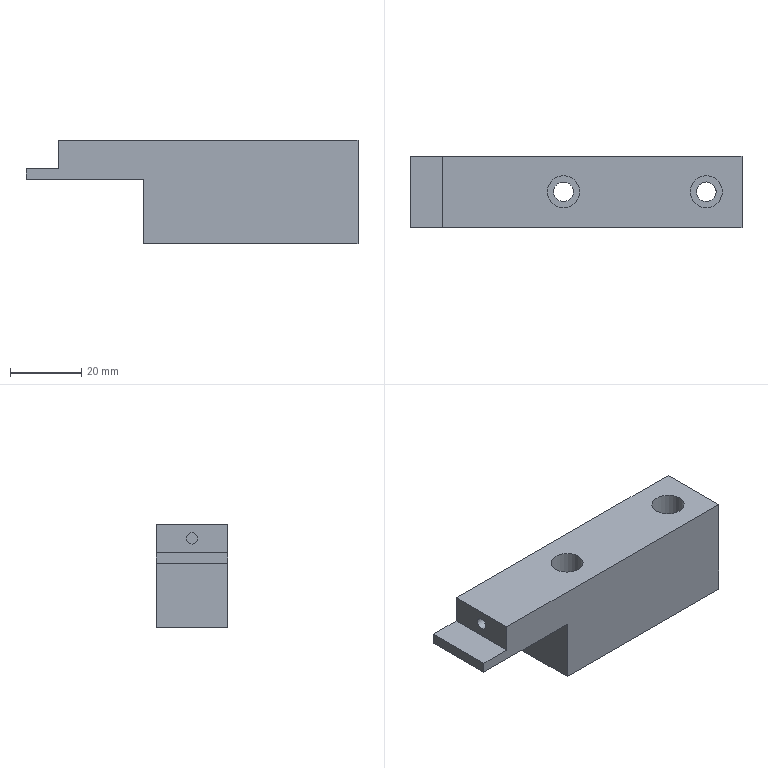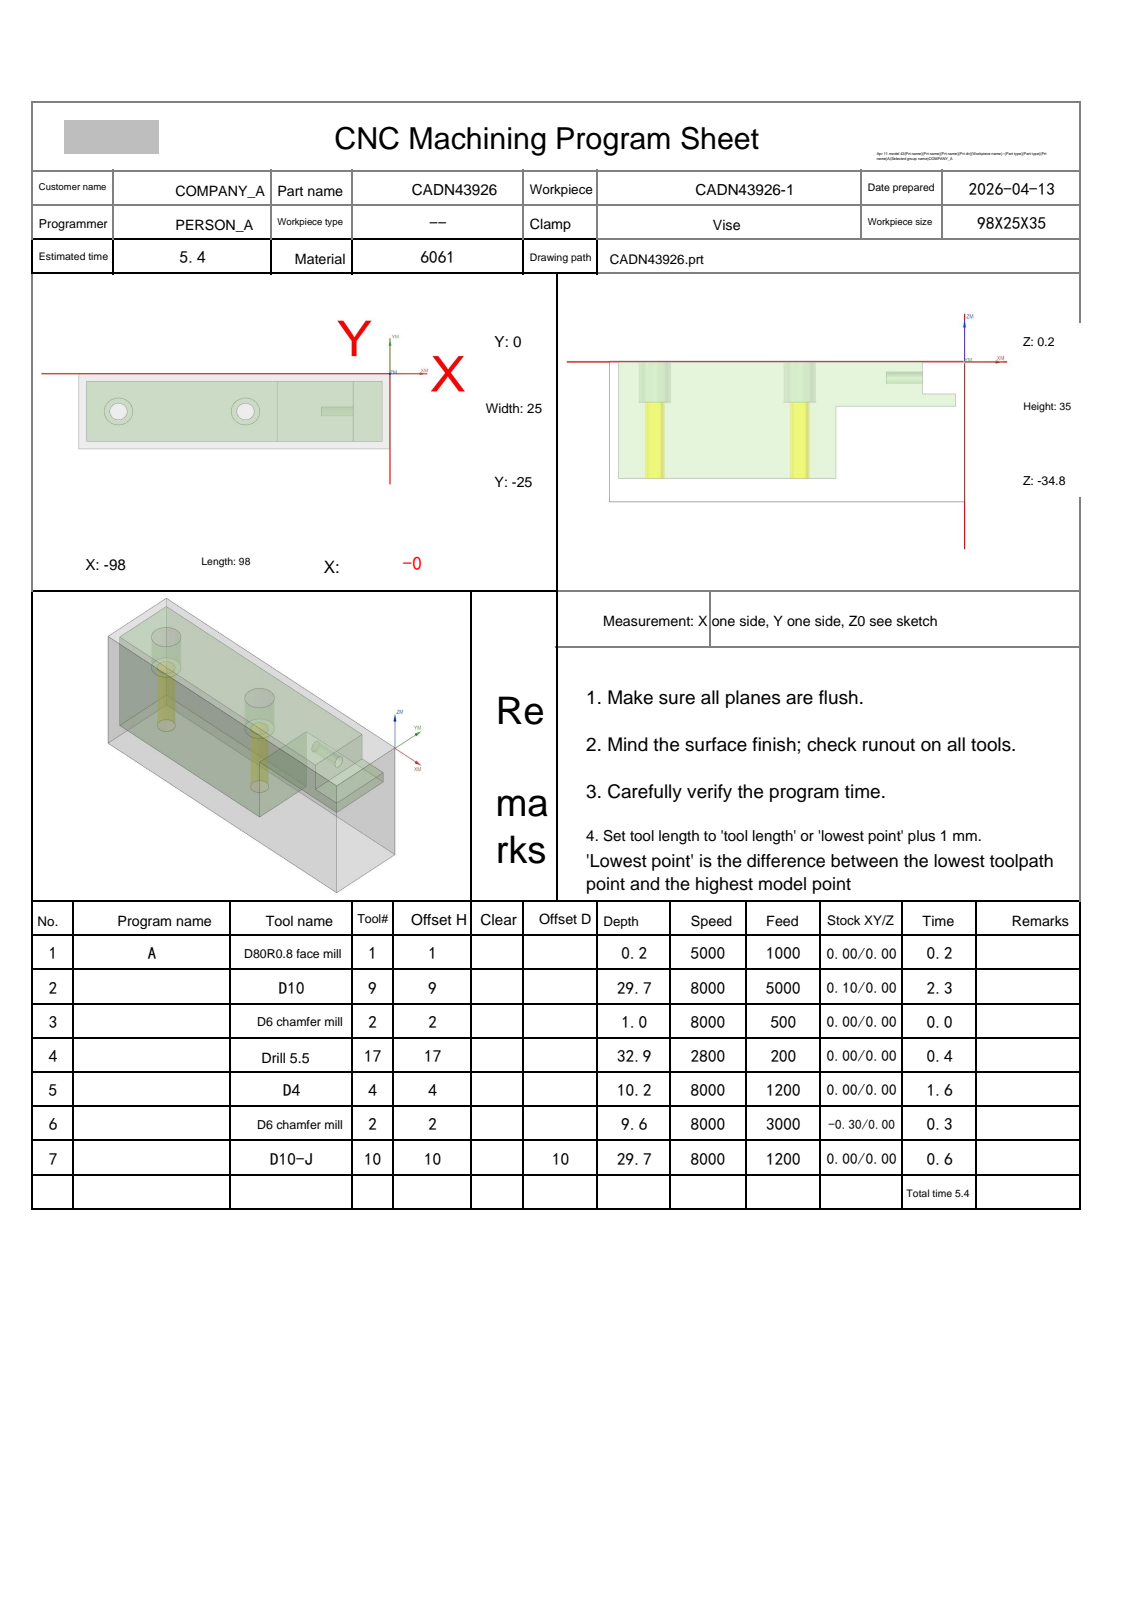NC program | NX | posted by the shop | part box 93 x 20 x 29 mm
Whole program:
%
O0001
(Machine time: 6.75 MIN)
(===Total Tool:6===)
(T1=D80R0.8 face mill D=80.  R=0.8  D-  H01 Z=0.    )
(T9=D10     D=10.  R=0.   D-  H09 Z=-29.5 )
(T2=D6 chamfer mill   D=6.   R=0.   D-  H02 Z=-9.45 )
(T17=drill 5.5  D=5.5  DR_a=118 D-  H17 Z=-32.65)
(T4=D4      D=4.   R=0.   D4  H04 Z=-10.  )
(T10=D10-J  D=10.  R=0.   D10 H10 Z=-29.5 )
G80 G90 G17 G49 G40
G91 G28 Z0
M01
N1 T01 M06
(D80R0.8 face mill  D=80. R=0.8 H=01 ce=0.00 di=0.00)
G00 G90 G54 X42.5 Y-12.5 M03 S5000
G43 H01 Z20.
M08
Z2.
G01 Z0.0 F1000.
X37.5
X-135.5
X-140.5
Z2.
G00 Z20.
G91 G28 Z0.0
M05
M09
G91 G28 Z0.0
M01
N2 T09 M06
(D10  D=10. R=0. H=09 ce=0.10 di=0.00)
G00 G90 G54 X-49. Y-27.6 M03 S8000
G43 H09 Z20.
M08
Z.5
G01 X-95.5 Z.358 F5000.
G02 X-100.6 Y-22.5 Z.333 I0.0 J5.1
G01 Y-2.5 Z.272
G02 X-95.5 Y2.6 Z.248 I5.1 J0.0
G01 X-2.5 Z-.037
G02 X2.6 Y-2.5 Z-.062 I0.0 J-5.1
G01 Y-22.5 Z-.123
G02 X-2.5 Y-27.6 Z-.147 I-5.1 J0.0
G01 X-95.5 Z-.432
G02 X-100.6 Y-22.5 Z-.456 I0.0 J5.1
G01 Y-2.5 Z-.517
G02 X-95.5 Y2.6 Z-.542 I5.1 J0.0
G01 X-2.5 Z-.826
G02 X2.6 Y-2.5 Z-.851 I0.0 J-5.1
G01 Y-22.5 Z-.912
G02 X-2.5 Y-27.6 Z-.937 I-5.1 J0.0
G01 X-95.5 Z-1.221
G02 X-100.6 Y-22.5 Z-1.246 I0.0 J5.1
G01 Y-2.5 Z-1.307
G02 X-95.5 Y2.6 Z-1.331 I5.1 J0.0
G01 X-2.5 Z-1.616
G02 X2.6 Y-2.5 Z-1.64 I0.0 J-5.1
G01 Y-22.5 Z-1.702
G02 X-2.5 Y-27.6 Z-1.726 I-5.1 J0.0
G01 X-95.5 Z-2.011
G02 X-100.6 Y-22.5 Z-2.035 I0.0 J5.1
G01 Y-2.5 Z-2.096
G02 X-95.5 Y2.6 Z-2.121 I5.1 J0.0
G01 X-2.5 Z-2.405
G02 X2.6 Y-2.5 Z-2.43 I0.0 J-5.1
G01 Y-22.5 Z-2.491
G02 X-2.5 Y-27.6 Z-2.516 I-5.1 J0.0
G01 X-95.5 Z-2.8
G02 X-100.6 Y-22.5 Z-2.825 I0.0 J5.1
G01 Y-2.5 Z-2.886
G02 X-95.5 Y2.6 Z-2.91 I5.1 J0.0
G01 X-2.5 Z-3.195
G02 X2.6 Y-2.5 Z-3.219 I0.0 J-5.1
G01 Y-22.5 Z-3.281
G02 X-2.5 Y-27.6 Z-3.305 I-5.1 J0.0
G01 X-95.5 Z-3.59
G02 X-100.6 Y-22.5 Z-3.614 I0.0 J5.1
G01 Y-2.5 Z-3.675
G02 X-95.5 Y2.6 Z-3.7 I5.1 J0.0
G01 X-2.5 Z-3.984
G02 X2.6 Y-2.5 Z-4.009 I0.0 J-5.1
G01 Y-22.5 Z-4.07
G02 X-2.5 Y-27.6 Z-4.095 I-5.1 J0.0
G01 X-95.5 Z-4.379
G02 X-100.6 Y-22.5 Z-4.404 I0.0 J5.1
G01 Y-2.5 Z-4.465
G02 X-95.5 Y2.6 Z-4.489 I5.1 J0.0
G01 X-2.5 Z-4.774
G02 X2.6 Y-2.5 Z-4.798 I0.0 J-5.1
G01 Y-22.5 Z-4.86
G02 X-2.5 Y-27.6 Z-4.884 I-5.1 J0.0
G01 X-95.5 Z-5.169
G02 X-100.6 Y-22.5 Z-5.193 I0.0 J5.1
G01 Y-2.5 Z-5.254
G02 X-95.5 Y2.6 Z-5.279 I5.1 J0.0
G01 X-2.5 Z-5.563
G02 X2.6 Y-2.5 Z-5.588 I0.0 J-5.1
G01 Y-22.5 Z-5.649
G02 X-2.5 Y-27.6 Z-5.674 I-5.1 J0.0
G01 X-95.5 Z-5.958
G02 X-100.6 Y-22.5 Z-5.983 I0.0 J5.1
G01 Y-2.5 Z-6.044
G02 X-95.5 Y2.6 Z-6.068 I5.1 J0.0
G01 X-2.5 Z-6.353
G02 X2.6 Y-2.5 Z-6.377 I0.0 J-5.1
G01 Y-22.5 Z-6.438
G02 X-2.5 Y-27.6 Z-6.463 I-5.1 J0.0
G01 X-95.5 Z-6.748
G02 X-100.6 Y-22.5 Z-6.772 I0.0 J5.1
G01 Y-2.5 Z-6.833
G02 X-95.5 Y2.6 Z-6.858 I5.1 J0.0
G01 X-2.5 Z-7.142
G02 X2.6 Y-2.5 Z-7.167 I0.0 J-5.1
G01 Y-22.5 Z-7.228
G02 X-2.5 Y-27.6 Z-7.252 I-5.1 J0.0
G01 X-95.5 Z-7.537
G02 X-100.6 Y-22.5 Z-7.562 I0.0 J5.1
G01 Y-2.5 Z-7.623
G02 X-95.5 Y2.6 Z-7.647 I5.1 J0.0
G01 X-2.5 Z-7.932
G02 X2.6 Y-2.5 Z-7.956 I0.0 J-5.1
G01 Y-22.5 Z-8.017
G02 X-2.5 Y-27.6 Z-8.042 I-5.1 J0.0
G01 X-95.5 Z-8.326
G02 X-100.6 Y-22.5 Z-8.351 I0.0 J5.1
G01 Y-2.5 Z-8.412
G02 X-95.5 Y2.6 Z-8.437 I5.1 J0.0
G01 X-2.5 Z-8.721
G02 X2.6 Y-2.5 Z-8.746 I0.0 J-5.1
G01 Y-22.5 Z-8.807
G02 X-2.5 Y-27.6 Z-8.831 I-5.1 J0.0
G01 X-95.5 Z-9.116
G02 X-100.6 Y-22.5 Z-9.14 I0.0 J5.1
G01 Y-2.5 Z-9.202
G02 X-95.5 Y2.6 Z-9.226 I5.1 J0.0
G01 X-2.5 Z-9.511
G02 X2.6 Y-2.5 Z-9.535 I0.0 J-5.1
G01 Y-22.5 Z-9.596
G02 X-2.5 Y-27.6 Z-9.621 I-5.1 J0.0
G01 X-95.5 Z-9.905
G02 X-100.6 Y-22.5 Z-9.93 I0.0 J5.1
G01 Y-2.5 Z-9.991
G02 X-95.5 Y2.6 Z-10.016 I5.1 J0.0
G01 X-2.5 Z-10.3
G02 X2.6 Y-2.5 Z-10.325 I0.0 J-5.1
G01 Y-22.5 Z-10.386
G02 X-2.5 Y-27.6 Z-10.41 I-5.1 J0.0
G01 X-95.5 Z-10.695
G02 X-100.6 Y-22.5 Z-10.719 I0.0 J5.1
G01 Y-2.5 Z-10.781
G02 X-95.5 Y2.6 Z-10.805 I5.1 J0.0
G01 X-2.5 Z-11.09
G02 X2.6 Y-2.5 Z-11.114 I0.0 J-5.1
G01 Y-22.5 Z-11.175
G02 X-2.5 Y-27.6 Z-11.2 I-5.1 J0.0
G01 X-95.5 Z-11.484
G02 X-100.6 Y-22.5 Z-11.509 I0.0 J5.1
G01 Y-2.5 Z-11.57
G02 X-95.5 Y2.6 Z-11.595 I5.1 J0.0
G01 X-2.5 Z-11.879
G02 X2.6 Y-2.5 Z-11.904 I0.0 J-5.1
G01 Y-22.5 Z-11.965
G02 X-2.5 Y-27.6 Z-11.989 I-5.1 J0.0
G01 X-95.5 Z-12.274
G02 X-100.6 Y-22.5 Z-12.298 I0.0 J5.1
G01 Y-2.5 Z-12.36
G02 X-95.5 Y2.6 Z-12.384 I5.1 J0.0
G01 X-2.5 Z-12.669
G02 X2.6 Y-2.5 Z-12.693 I0.0 J-5.1
G01 Y-22.5 Z-12.754
G02 X-2.5 Y-27.6 Z-12.779 I-5.1 J0.0
G01 X-95.5 Z-13.063
G02 X-100.6 Y-22.5 Z-13.088 I0.0 J5.1
G01 Y-2.5 Z-13.149
G02 X-95.5 Y2.6 Z-13.174 I5.1 J0.0
G01 X-2.5 Z-13.458
G02 X2.6 Y-2.5 Z-13.483 I0.0 J-5.1
G01 Y-22.5 Z-13.544
G02 X-2.5 Y-27.6 Z-13.568 I-5.1 J0.0
G01 X-95.5 Z-13.853
G02 X-100.6 Y-22.5 Z-13.877 I0.0 J5.1
G01 Y-2.5 Z-13.938
G02 X-95.5 Y2.6 Z-13.963 I5.1 J0.0
G01 X-2.5 Z-14.248
G02 X2.6 Y-2.5 Z-14.272 I0.0 J-5.1
G01 Y-22.5 Z-14.333
G02 X-2.5 Y-27.6 Z-14.358 I-5.1 J0.0
G01 X-95.5 Z-14.642
G02 X-100.6 Y-22.5 Z-14.667 I0.0 J5.1
G01 Y-2.5 Z-14.728
G02 X-95.5 Y2.6 Z-14.752 I5.1 J0.0
G01 X-2.5 Z-15.037
G02 X2.6 Y-2.5 Z-15.062 I0.0 J-5.1
G01 Y-22.5 Z-15.123
G02 X-2.5 Y-27.6 Z-15.147 I-5.1 J0.0
G01 X-95.5 Z-15.432
G02 X-100.6 Y-22.5 Z-15.456 I0.0 J5.1
G01 Y-2.5 Z-15.517
G02 X-95.5 Y2.6 Z-15.542 I5.1 J0.0
G01 X-2.5 Z-15.826
G02 X2.6 Y-2.5 Z-15.851 I0.0 J-5.1
G01 Y-22.5 Z-15.912
G02 X-2.5 Y-27.6 Z-15.937 I-5.1 J0.0
G01 X-95.5 Z-16.221
G02 X-100.6 Y-22.5 Z-16.246 I0.0 J5.1
G01 Y-2.5 Z-16.307
G02 X-95.5 Y2.6 Z-16.331 I5.1 J0.0
G01 X-2.5 Z-16.616
G02 X2.6 Y-2.5 Z-16.64 I0.0 J-5.1
G01 Y-22.5 Z-16.702
G02 X-2.5 Y-27.6 Z-16.726 I-5.1 J0.0
G01 X-95.5 Z-17.011
G02 X-100.6 Y-22.5 Z-17.035 I0.0 J5.1
G01 Y-2.5 Z-17.096
G02 X-95.5 Y2.6 Z-17.121 I5.1 J0.0
G01 X-2.5 Z-17.405
G02 X2.6 Y-2.5 Z-17.43 I0.0 J-5.1
G01 Y-22.5 Z-17.491
G02 X-2.5 Y-27.6 Z-17.516 I-5.1 J0.0
G01 X-95.5 Z-17.8
G02 X-100.6 Y-22.5 Z-17.825 I0.0 J5.1
G01 Y-2.5 Z-17.886
G02 X-95.5 Y2.6 Z-17.91 I5.1 J0.0
G01 X-2.5 Z-18.195
G02 X2.6 Y-2.5 Z-18.219 I0.0 J-5.1
G01 Y-22.5 Z-18.281
G02 X-2.5 Y-27.6 Z-18.305 I-5.1 J0.0
G01 X-95.5 Z-18.59
G02 X-100.6 Y-22.5 Z-18.614 I0.0 J5.1
G01 Y-2.5 Z-18.675
G02 X-95.5 Y2.6 Z-18.7 I5.1 J0.0
G01 X-2.5 Z-18.984
G02 X2.6 Y-2.5 Z-19.009 I0.0 J-5.1
G01 Y-22.5 Z-19.07
G02 X-2.5 Y-27.6 Z-19.095 I-5.1 J0.0
G01 X-95.5 Z-19.379
G02 X-100.6 Y-22.5 Z-19.404 I0.0 J5.1
G01 Y-2.5 Z-19.465
G02 X-95.5 Y2.6 Z-19.489 I5.1 J0.0
G01 X-2.5 Z-19.774
G02 X2.6 Y-2.5 Z-19.798 I0.0 J-5.1
G01 Y-22.5 Z-19.86
G02 X-2.5 Y-27.6 Z-19.884 I-5.1 J0.0
G01 X-95.5 Z-20.169
G02 X-100.6 Y-22.5 Z-20.193 I0.0 J5.1
G01 Y-2.5 Z-20.254
G02 X-95.5 Y2.6 Z-20.279 I5.1 J0.0
G01 X-2.5 Z-20.563
G02 X2.6 Y-2.5 Z-20.588 I0.0 J-5.1
G01 Y-22.5 Z-20.649
G02 X-2.5 Y-27.6 Z-20.674 I-5.1 J0.0
G01 X-95.5 Z-20.958
G02 X-100.6 Y-22.5 Z-20.983 I0.0 J5.1
G01 Y-2.5 Z-21.044
G02 X-95.5 Y2.6 Z-21.068 I5.1 J0.0
G01 X-2.5 Z-21.353
G02 X2.6 Y-2.5 Z-21.377 I0.0 J-5.1
G01 Y-22.5 Z-21.438
G02 X-2.5 Y-27.6 Z-21.463 I-5.1 J0.0
G01 X-95.5 Z-21.748
G02 X-100.6 Y-22.5 Z-21.772 I0.0 J5.1
G01 Y-2.5 Z-21.833
G02 X-95.5 Y2.6 Z-21.858 I5.1 J0.0
G01 X-2.5 Z-22.142
G02 X2.6 Y-2.5 Z-22.167 I0.0 J-5.1
G01 Y-22.5 Z-22.228
G02 X-2.5 Y-27.6 Z-22.252 I-5.1 J0.0
G01 X-95.5 Z-22.537
G02 X-100.6 Y-22.5 Z-22.562 I0.0 J5.1
G01 Y-2.5 Z-22.623
G02 X-95.5 Y2.6 Z-22.647 I5.1 J0.0
G01 X-2.5 Z-22.932
G02 X2.6 Y-2.5 Z-22.956 I0.0 J-5.1
G01 Y-22.5 Z-23.017
G02 X-2.5 Y-27.6 Z-23.042 I-5.1 J0.0
G01 X-95.5 Z-23.326
G02 X-100.6 Y-22.5 Z-23.351 I0.0 J5.1
G01 Y-2.5 Z-23.412
G02 X-95.5 Y2.6 Z-23.437 I5.1 J0.0
G01 X-2.5 Z-23.721
G02 X2.6 Y-2.5 Z-23.746 I0.0 J-5.1
G01 Y-22.5 Z-23.807
G02 X-2.5 Y-27.6 Z-23.831 I-5.1 J0.0
G01 X-95.5 Z-24.116
G02 X-100.6 Y-22.5 Z-24.14 I0.0 J5.1
G01 Y-2.5 Z-24.202
G02 X-95.5 Y2.6 Z-24.226 I5.1 J0.0
G01 X-2.5 Z-24.511
G02 X2.6 Y-2.5 Z-24.535 I0.0 J-5.1
G01 Y-22.5 Z-24.596
G02 X-2.5 Y-27.6 Z-24.621 I-5.1 J0.0
G01 X-95.5 Z-24.905
G02 X-100.6 Y-22.5 Z-24.93 I0.0 J5.1
G01 Y-2.5 Z-24.991
G02 X-95.5 Y2.6 Z-25.016 I5.1 J0.0
G01 X-2.5 Z-25.3
G02 X2.6 Y-2.5 Z-25.325 I0.0 J-5.1
G01 Y-22.5 Z-25.386
G02 X-2.5 Y-27.6 Z-25.41 I-5.1 J0.0
G01 X-95.5 Z-25.695
G02 X-100.6 Y-22.5 Z-25.719 I0.0 J5.1
G01 Y-2.5 Z-25.781
G02 X-95.5 Y2.6 Z-25.805 I5.1 J0.0
G01 X-2.5 Z-26.09
G02 X2.6 Y-2.5 Z-26.114 I0.0 J-5.1
G01 Y-22.5 Z-26.175
G02 X-2.5 Y-27.6 Z-26.2 I-5.1 J0.0
G01 X-95.5 Z-26.484
G02 X-100.6 Y-22.5 Z-26.509 I0.0 J5.1
G01 Y-2.5 Z-26.57
G02 X-95.5 Y2.6 Z-26.595 I5.1 J0.0
G01 X-2.5 Z-26.879
G02 X2.6 Y-2.5 Z-26.904 I0.0 J-5.1
G01 Y-22.5 Z-26.965
G02 X-2.5 Y-27.6 Z-26.989 I-5.1 J0.0
G01 X-95.5 Z-27.274
G02 X-100.6 Y-22.5 Z-27.298 I0.0 J5.1
G01 Y-2.5 Z-27.36
G02 X-95.5 Y2.6 Z-27.384 I5.1 J0.0
G01 X-2.5 Z-27.669
G02 X2.6 Y-2.5 Z-27.693 I0.0 J-5.1
G01 Y-22.5 Z-27.754
G02 X-2.5 Y-27.6 Z-27.779 I-5.1 J0.0
G01 X-95.5 Z-28.063
G02 X-100.6 Y-22.5 Z-28.088 I0.0 J5.1
G01 Y-2.5 Z-28.149
G02 X-95.5 Y2.6 Z-28.174 I5.1 J0.0
G01 X-2.5 Z-28.458
G02 X2.6 Y-2.5 Z-28.483 I0.0 J-5.1
G01 Y-22.5 Z-28.544
G02 X-2.5 Y-27.6 Z-28.568 I-5.1 J0.0
G01 X-95.5 Z-28.853
G02 X-100.6 Y-22.5 Z-28.877 I0.0 J5.1
G01 Y-2.5 Z-28.938
G02 X-95.5 Y2.6 Z-28.963 I5.1 J0.0
G01 X-2.5 Z-29.248
G02 X2.6 Y-2.5 Z-29.272 I0.0 J-5.1
G01 Y-22.5 Z-29.333
G02 X-2.5 Y-27.6 Z-29.358 I-5.1 J0.0
G01 X-49. Z-29.5
X-95.5
G02 X-100.6 Y-22.5 I0.0 J5.1
G01 Y-2.5
G02 X-95.5 Y2.6 I5.1 J0.0
G01 X-2.5
G02 X2.6 Y-2.5 I0.0 J-5.1
G01 Y-22.5
G02 X-2.5 Y-27.6 I-5.1 J0.0
G01 X-49.
X-49.5
Z-28.5
G00 Z20.
G00 G90 X5.5 Y-12.5 M03 S6000
Z20.
Z.009
G01 Z-.491 F3500.
X-1.5
Y-1.5
X-6.5
Y-23.5
X-1.5
Y-12.5
Y-12.
Z.009
G00 Z.5
X5.5 Y-12.5
Z-.481
G01 Z-.981
X-1.5
Y-1.5
X-6.5
Y-23.5
X-1.5
Y-12.5
Y-12.
Z-.481
G00 Z.009
X5.5 Y-12.5
Z-.972
G01 Z-1.472
X-1.5
Y-1.5
X-6.5
Y-23.5
X-1.5
Y-12.5
Y-12.
Z-.972
G00 Z-.481
X5.5 Y-12.5
Z-1.463
G01 Z-1.963
X-1.5
Y-1.5
X-6.5
Y-23.5
X-1.5
Y-12.5
Y-12.
Z-1.463
G00 Z-.972
X5.5 Y-12.5
Z-1.953
G01 Z-2.453
X-1.5
Y-1.5
X-6.5
Y-23.5
X-1.5
Y-12.5
Y-12.
Z-1.953
G00 Z-1.463
X5.5 Y-12.5
Z-2.444
G01 Z-2.944
X-1.5
Y-1.5
X-6.5
Y-23.5
X-1.5
Y-12.5
Y-12.
Z-2.444
G00 Z-1.953
X5.5 Y-12.5
Z-2.934
G01 Z-3.434
X-1.5
Y-1.5
X-6.5
Y-23.5
X-1.5
Y-12.5
Y-12.
Z-2.934
G00 Z-2.444
X5.5 Y-12.5
Z-3.425
G01 Z-3.925
X-1.5
Y-1.5
X-6.5
Y-23.5
X-1.5
Y-12.5
Y-12.
Z-3.425
G00 Z-2.934
X5.5 Y-12.5
Z-3.916
G01 Z-4.416
X-1.5
Y-1.5
X-6.5
Y-23.5
X-1.5
Y-12.5
Y-12.
Z-3.916
G00 Z-3.425
X5.5 Y-12.5
Z-4.406
G01 Z-4.906
X-1.5
Y-1.5
X-6.5
Y-23.5
X-1.5
Y-12.5
Y-12.
Z-4.406
G00 Z-3.916
X5.5 Y-12.5
Z-4.897
G01 Z-5.397
X-1.5
Y-1.5
X-6.5
Y-23.5
X-1.5
Y-12.5
Y-12.
Z-4.897
G00 Z-4.406
X5.5 Y-12.5
Z-5.388
G01 Z-5.888
X-1.5
Y-1.5
X-6.5
Y-23.5
X-1.5
Y-12.5
Y-12.
Z-5.388
G00 Z-4.897
X5.5 Y-12.5
Z-5.878
G01 Z-6.378
X-1.5
Y-1.5
X-6.5
Y-23.5
X-1.5
Y-12.5
Y-12.
Z-5.878
G00 Z-5.388
X5.5 Y-12.5
Z-6.369
G01 Z-6.869
X-1.5
Y-1.5
X-6.5
Y-23.5
X-1.5
Y-12.5
Y-12.
Z-6.369
G00 Z-5.878
X5.5 Y-12.5
Z-6.859
G01 Z-7.359
X-1.5
Y-1.5
X-6.5
Y-23.5
X-1.5
Y-12.5
Y-12.
Z-6.859
G00 Z-6.369
X5.5 Y-12.5
Z-7.35
G01 Z-7.85
X-1.5
Y-1.5
X-6.5
Y-23.5
X-1.5
Y-12.5
Y-12.
Z-7.35
G00 Z20.
G91 G28 Z0.0
M05
M09
G91 G28 Z0.0
M01
N3 T02 M06
(D6 chamfer mill  D=6. R=0. H=02 ce=0.00 di=0.10)
G00 G90 G54 X-85.5 Y-12.55 M03 S8000
G43 H02 Z20.
M08
G98 G81 X-85.5 Y-12.55 Z-.8 R1. F500.
X-45.5
G80
G00 Z20.
G91 G28 Z0.0
M05
M09
G91 G28 Z0.0
M01
N4 T17 M06
(Drill 5.5 D=5.5 DR_a=118 H=17)
G00 G90 G54 X-85.5 Y-12.55 M03 S2800
G43 H17 Z20.
M08
G98 G83 X-85.5 Y-12.55 Z-32.652 R1. F200. Q2.
X-45.5
G80
G00 Z20.
G91 G28 Z0.0
M05
M09
G91 G28 Z0.0
M01
N5 T04 M06
(D4  D=4. R=0. H=04 ce=0.10 di=0.00)
G00 G90 G54 X-85.5 Y-12.55 M03 S8000
G43 H04 Z20.
M08
Z.5
G03 X-86.1 Y-11.95 I-.6 J0.0 F1200.
X-86.7 Y-12.55 I0.0 J-.6
X-86.7 Y-12.55 Z.2 I1.2 J0.0
X-86.7 Y-12.55 Z-.1 I1.2 J0.0
X-86.7 Y-12.55 Z-.4 I1.2 J0.0
X-86.7 Y-12.55 Z-.7 I1.2 J0.0
X-86.7 Y-12.55 Z-1. I1.2 J0.0
X-86.7 Y-12.55 Z-1.3 I1.2 J0.0
X-86.7 Y-12.55 Z-1.6 I1.2 J0.0
X-86.7 Y-12.55 Z-1.9 I1.2 J0.0
X-86.7 Y-12.55 Z-2.2 I1.2 J0.0
X-86.7 Y-12.55 Z-2.5 I1.2 J0.0
X-86.7 Y-12.55 Z-2.8 I1.2 J0.0
X-86.7 Y-12.55 Z-3.1 I1.2 J0.0
X-86.7 Y-12.55 Z-3.4 I1.2 J0.0
X-86.7 Y-12.55 Z-3.7 I1.2 J0.0
X-86.7 Y-12.55 Z-4. I1.2 J0.0
X-86.7 Y-12.55 Z-4.3 I1.2 J0.0
X-86.7 Y-12.55 Z-4.6 I1.2 J0.0
X-86.7 Y-12.55 Z-4.9 I1.2 J0.0
X-86.7 Y-12.55 Z-5.2 I1.2 J0.0
X-86.7 Y-12.55 Z-5.5 I1.2 J0.0
X-86.7 Y-12.55 Z-5.8 I1.2 J0.0
X-86.7 Y-12.55 Z-6.1 I1.2 J0.0
X-86.7 Y-12.55 Z-6.4 I1.2 J0.0
X-86.7 Y-12.55 Z-6.7 I1.2 J0.0
X-86.7 Y-12.55 Z-7. I1.2 J0.0
X-86.7 Y-12.55 Z-7.3 I1.2 J0.0
X-86.7 Y-12.55 Z-7.6 I1.2 J0.0
X-86.7 Y-12.55 Z-7.9 I1.2 J0.0
X-86.7 Y-12.55 Z-8.2 I1.2 J0.0
X-86.7 Y-12.55 Z-8.5 I1.2 J0.0
X-86.7 Y-12.55 Z-8.8 I1.2 J0.0
X-86.7 Y-12.55 Z-9.1 I1.2 J0.0
X-86.7 Y-12.55 Z-9.4 I1.2 J0.0
X-86.7 Y-12.55 Z-9.7 I1.2 J0.0
X-86.7 Y-12.55 Z-10. I1.2 J0.0
X-85.5 Y-13.75 I1.2 J0.0
X-84.3 Y-12.55 I0.0 J1.2
X-85.5 Y-11.35 I-1.2 J0.0
X-86.7 Y-12.55 I0.0 J-1.2
X-86.1 Y-13.15 I.6 J0.0
X-85.5 Y-12.55 I0.0 J.6
G00 Z.5
G03 X-86.7 Y-11.35 I-1.2 J0.0
X-87.9 Y-12.55 I0.0 J-1.2
X-87.9 Y-12.55 Z.2 I2.4 J0.0
X-87.9 Y-12.55 Z-.1 I2.4 J0.0
X-87.9 Y-12.55 Z-.4 I2.4 J0.0
X-87.9 Y-12.55 Z-.7 I2.4 J0.0
X-87.9 Y-12.55 Z-1. I2.4 J0.0
X-87.9 Y-12.55 Z-1.3 I2.4 J0.0
X-87.9 Y-12.55 Z-1.6 I2.4 J0.0
X-87.9 Y-12.55 Z-1.9 I2.4 J0.0
X-87.9 Y-12.55 Z-2.2 I2.4 J0.0
X-87.9 Y-12.55 Z-2.5 I2.4 J0.0
X-87.9 Y-12.55 Z-2.8 I2.4 J0.0
X-87.9 Y-12.55 Z-3.1 I2.4 J0.0
X-87.9 Y-12.55 Z-3.4 I2.4 J0.0
X-87.9 Y-12.55 Z-3.7 I2.4 J0.0
X-87.9 Y-12.55 Z-4. I2.4 J0.0
X-87.9 Y-12.55 Z-4.3 I2.4 J0.0
X-87.9 Y-12.55 Z-4.6 I2.4 J0.0
X-87.9 Y-12.55 Z-4.9 I2.4 J0.0
X-87.9 Y-12.55 Z-5.2 I2.4 J0.0
X-87.9 Y-12.55 Z-5.5 I2.4 J0.0
X-87.9 Y-12.55 Z-5.8 I2.4 J0.0
X-87.9 Y-12.55 Z-6.1 I2.4 J0.0
X-87.9 Y-12.55 Z-6.4 I2.4 J0.0
X-87.9 Y-12.55 Z-6.7 I2.4 J0.0
X-87.9 Y-12.55 Z-7. I2.4 J0.0
X-87.9 Y-12.55 Z-7.3 I2.4 J0.0
X-87.9 Y-12.55 Z-7.6 I2.4 J0.0
X-87.9 Y-12.55 Z-7.9 I2.4 J0.0
X-87.9 Y-12.55 Z-8.2 I2.4 J0.0
X-87.9 Y-12.55 Z-8.5 I2.4 J0.0
X-87.9 Y-12.55 Z-8.8 I2.4 J0.0
X-87.9 Y-12.55 Z-9.1 I2.4 J0.0
X-87.9 Y-12.55 Z-9.4 I2.4 J0.0
X-87.9 Y-12.55 Z-9.7 I2.4 J0.0
X-87.9 Y-12.55 Z-10. I2.4 J0.0
X-85.5 Y-14.95 I2.4 J0.0
X-83.1 Y-12.55 I0.0 J2.4
X-85.5 Y-10.15 I-2.4 J0.0
X-87.9 Y-12.55 I0.0 J-2.4
X-86.7 Y-13.75 I1.2 J0.0
X-85.5 Y-12.55 I0.0 J1.2
G00 Z20.
X-45.5
Z.5
G03 X-46.1 Y-11.95 I-.6 J0.0
X-46.7 Y-12.55 I0.0 J-.6
X-46.7 Y-12.55 Z.2 I1.2 J0.0
X-46.7 Y-12.55 Z-.1 I1.2 J0.0
X-46.7 Y-12.55 Z-.4 I1.2 J0.0
X-46.7 Y-12.55 Z-.7 I1.2 J0.0
X-46.7 Y-12.55 Z-1. I1.2 J0.0
X-46.7 Y-12.55 Z-1.3 I1.2 J0.0
X-46.7 Y-12.55 Z-1.6 I1.2 J0.0
X-46.7 Y-12.55 Z-1.9 I1.2 J0.0
X-46.7 Y-12.55 Z-2.2 I1.2 J0.0
X-46.7 Y-12.55 Z-2.5 I1.2 J0.0
X-46.7 Y-12.55 Z-2.8 I1.2 J0.0
X-46.7 Y-12.55 Z-3.1 I1.2 J0.0
X-46.7 Y-12.55 Z-3.4 I1.2 J0.0
X-46.7 Y-12.55 Z-3.7 I1.2 J0.0
X-46.7 Y-12.55 Z-4. I1.2 J0.0
X-46.7 Y-12.55 Z-4.3 I1.2 J0.0
X-46.7 Y-12.55 Z-4.6 I1.2 J0.0
X-46.7 Y-12.55 Z-4.9 I1.2 J0.0
X-46.7 Y-12.55 Z-5.2 I1.2 J0.0
X-46.7 Y-12.55 Z-5.5 I1.2 J0.0
X-46.7 Y-12.55 Z-5.8 I1.2 J0.0
X-46.7 Y-12.55 Z-6.1 I1.2 J0.0
X-46.7 Y-12.55 Z-6.4 I1.2 J0.0
X-46.7 Y-12.55 Z-6.7 I1.2 J0.0
X-46.7 Y-12.55 Z-7. I1.2 J0.0
X-46.7 Y-12.55 Z-7.3 I1.2 J0.0
X-46.7 Y-12.55 Z-7.6 I1.2 J0.0
X-46.7 Y-12.55 Z-7.9 I1.2 J0.0
X-46.7 Y-12.55 Z-8.2 I1.2 J0.0
X-46.7 Y-12.55 Z-8.5 I1.2 J0.0
X-46.7 Y-12.55 Z-8.8 I1.2 J0.0
X-46.7 Y-12.55 Z-9.1 I1.2 J0.0
X-46.7 Y-12.55 Z-9.4 I1.2 J0.0
X-46.7 Y-12.55 Z-9.7 I1.2 J0.0
X-46.7 Y-12.55 Z-10. I1.2 J0.0
X-45.5 Y-13.75 I1.2 J0.0
X-44.3 Y-12.55 I0.0 J1.2
X-45.5 Y-11.35 I-1.2 J0.0
X-46.7 Y-12.55 I0.0 J-1.2
X-46.1 Y-13.15 I.6 J0.0
X-45.5 Y-12.55 I0.0 J.6
G00 Z.5
G03 X-46.7 Y-11.35 I-1.2 J0.0
X-47.9 Y-12.55 I0.0 J-1.2
X-47.9 Y-12.55 Z.2 I2.4 J0.0
X-47.9 Y-12.55 Z-.1 I2.4 J0.0
X-47.9 Y-12.55 Z-.4 I2.4 J0.0
X-47.9 Y-12.55 Z-.7 I2.4 J0.0
X-47.9 Y-12.55 Z-1. I2.4 J0.0
X-47.9 Y-12.55 Z-1.3 I2.4 J0.0
X-47.9 Y-12.55 Z-1.6 I2.4 J0.0
X-47.9 Y-12.55 Z-1.9 I2.4 J0.0
X-47.9 Y-12.55 Z-2.2 I2.4 J0.0
X-47.9 Y-12.55 Z-2.5 I2.4 J0.0
X-47.9 Y-12.55 Z-2.8 I2.4 J0.0
X-47.9 Y-12.55 Z-3.1 I2.4 J0.0
X-47.9 Y-12.55 Z-3.4 I2.4 J0.0
X-47.9 Y-12.55 Z-3.7 I2.4 J0.0
X-47.9 Y-12.55 Z-4. I2.4 J0.0
X-47.9 Y-12.55 Z-4.3 I2.4 J0.0
X-47.9 Y-12.55 Z-4.6 I2.4 J0.0
X-47.9 Y-12.55 Z-4.9 I2.4 J0.0
X-47.9 Y-12.55 Z-5.2 I2.4 J0.0
X-47.9 Y-12.55 Z-5.5 I2.4 J0.0
X-47.9 Y-12.55 Z-5.8 I2.4 J0.0
X-47.9 Y-12.55 Z-6.1 I2.4 J0.0
X-47.9 Y-12.55 Z-6.4 I2.4 J0.0
X-47.9 Y-12.55 Z-6.7 I2.4 J0.0
X-47.9 Y-12.55 Z-7. I2.4 J0.0
X-47.9 Y-12.55 Z-7.3 I2.4 J0.0
X-47.9 Y-12.55 Z-7.6 I2.4 J0.0
X-47.9 Y-12.55 Z-7.9 I2.4 J0.0
X-47.9 Y-12.55 Z-8.2 I2.4 J0.0
X-47.9 Y-12.55 Z-8.5 I2.4 J0.0
X-47.9 Y-12.55 Z-8.8 I2.4 J0.0
X-47.9 Y-12.55 Z-9.1 I2.4 J0.0
X-47.9 Y-12.55 Z-9.4 I2.4 J0.0
X-47.9 Y-12.55 Z-9.7 I2.4 J0.0
X-47.9 Y-12.55 Z-10. I2.4 J0.0
X-45.5 Y-14.95 I2.4 J0.0
X-43.1 Y-12.55 I0.0 J2.4
X-45.5 Y-10.15 I-2.4 J0.0
X-47.9 Y-12.55 I0.0 J-2.4
X-46.7 Y-13.75 I1.2 J0.0
X-45.5 Y-12.55 I0.0 J1.2
G00 Z20.
G00 G90 X-85.5 Y-12.55 M03 S8000
Z20.
Z.5
G41 D04
G01 X-85.532 Y-12.353 F500.
G03 X-86.758 Y-11.308 I-1.226 J-.197
X-88. Y-12.55 I0.0 J-1.242
X-88. Y-12.55 Z-4.5 I2.5 J0.0
X-88. Y-12.55 Z-9.5 I2.5 J0.0
X-87.523 Y-14.019 Z-10. I2.5 J0.0
X-85.5 Y-15.05 I2.023 J1.469
X-83. Y-12.55 I0.0 J2.5
X-85.5 Y-10.05 I-2.5 J0.0
X-88. Y-12.55 I0.0 J-2.5
X-87.523 Y-14.019 I2.5 J0.0
X-86.518 Y-14.531 I1.005 J.73
X-85.276 Y-13.289 I0.0 J1.242
X-85.41 Y-12.728 I-1.242 J0.0
G01 G40 X-85.5 Y-12.55
G00 Z20.
X-45.5
Z.5
G41 D04
G01 X-45.532 Y-12.353
G03 X-46.758 Y-11.308 I-1.226 J-.197
X-48. Y-12.55 I0.0 J-1.242
X-48. Y-12.55 Z-4.5 I2.5 J0.0
X-48. Y-12.55 Z-9.5 I2.5 J0.0
X-47.523 Y-14.019 Z-10. I2.5 J0.0
X-45.5 Y-15.05 I2.023 J1.469
X-43. Y-12.55 I0.0 J2.5
X-45.5 Y-10.05 I-2.5 J0.0
X-48. Y-12.55 I0.0 J-2.5
X-47.523 Y-14.019 I2.5 J0.0
X-46.518 Y-14.531 I1.005 J.73
X-45.276 Y-13.289 I0.0 J1.242
X-45.41 Y-12.728 I-1.242 J0.0
G01 G40 X-45.5 Y-12.55
G00 Z20.
G91 G28 Z0.0
M05
M09
G91 G28 Z0.0
M01
N6 T02 M06
(D6 chamfer mill  D=6. R=0. H=02 ce=0.00 di=0.00)
G00 G90 G54 X-53.3 Y-24.628 M03 S8000
G43 H02 Z20.
M08
Z2.099
G01 Z-1.499 F3000.
G03 X-53.22 Y-24.328 I-.52 J.3
X-53.52 Y-23.808 I-.6 J0.0
G01 X-53.55 Y-23.8
X-95.5
G02 X-96.8 Y-22.5 I0.0 J1.3
G01 Y-2.5
G02 X-95.5 Y-1.2 I1.3 J0.0
G01 X-11.6
G02 X-10.3 Y-2.5 I0.0 J-1.3
G01 Y-22.5
G02 X-11.6 Y-23.8 I-1.3 J0.0
G01 X-53.55
X-53.58 Y-23.808
G03 X-53.88 Y-24.328 I.3 J-.52
X-53.8 Y-24.628 I.6 J0.0
G01 Z2.099
G00 Z20.
X-8.544 Y-.372
Z1.755
G01 Z-9.449
G03 X-8.624 Y-.672 I.52 J-.3
X-8.324 Y-1.192 I.6 J0.0
G01 X-8.294 Y-1.2
X-2.5
G02 X-1.2 Y-2.5 I0.0 J-1.3
G01 Y-22.5
G02 X-2.5 Y-23.8 I-1.3 J0.0
G01 X-8.328
X-8.355 Y-23.807
G03 X-8.625 Y-24.275 I.27 J-.468
X-8.553 Y-24.545 I.54 J0.0
G01 Z1.755
G00 Z20.
G00 G90 X-88.609 Y-14.731 M03 S8000
Z20.
Z2.5
G01 X-88.477 Y-14.917 Z2.417 F500.
X-88.194 Y-15.234 Z2.262
X-87.877 Y-15.518 Z2.107
X-87.531 Y-15.765 Z1.953
X-87.269 Y-15.916 Z1.843
X-86.882 Y-16.093 Z1.688
X-86.478 Y-16.225 Z1.533
X-86.061 Y-16.311 Z1.378
X-85.637 Y-16.351 Z1.223
X-85.212 Y-16.342 Z1.068
X-84.79 Y-16.286 Z.913
X-84.377 Y-16.183 Z.758
X-83.978 Y-16.035 Z.604
X-83.599 Y-15.843 Z.449
X-83.242 Y-15.61 Z.294
X-82.915 Y-15.339 Z.139
X-82.619 Y-15.033 Z-.016
X-82.36 Y-14.696 Z-.171
X-82.14 Y-14.331 Z-.326
X-81.962 Y-13.945 Z-.48
X-81.828 Y-13.541 Z-.635
X-81.741 Y-13.125 Z-.79
X-81.7 Y-12.701 Z-.945
Y-12.55 Z-1.
G03 X-85.5 Y-8.75 I-3.8 J0.0
X-89.3 Y-12.55 I0.0 J-3.8
X-85.5 Y-16.35 I3.8 J0.0
X-81.7 Y-12.55 I0.0 J3.8
X-81.733 Y-12.051 I-3.8 J0.0
G01 Z1.5
G00 Z20.
X-48.609 Y-14.731
Z2.5
G01 X-48.477 Y-14.917 Z2.417
X-48.194 Y-15.234 Z2.262
X-47.877 Y-15.518 Z2.107
X-47.531 Y-15.765 Z1.953
X-47.269 Y-15.916 Z1.843
X-46.882 Y-16.093 Z1.688
X-46.478 Y-16.225 Z1.533
X-46.061 Y-16.311 Z1.378
X-45.637 Y-16.351 Z1.223
X-45.212 Y-16.342 Z1.068
X-44.79 Y-16.286 Z.913
X-44.377 Y-16.183 Z.758
X-43.978 Y-16.035 Z.604
X-43.599 Y-15.843 Z.449
X-43.242 Y-15.61 Z.294
X-42.915 Y-15.339 Z.139
X-42.619 Y-15.033 Z-.016
X-42.36 Y-14.696 Z-.171
X-42.14 Y-14.331 Z-.326
X-41.962 Y-13.945 Z-.48
X-41.828 Y-13.541 Z-.635
X-41.741 Y-13.125 Z-.79
X-41.7 Y-12.701 Z-.945
Y-12.55 Z-1.
G03 X-45.5 Y-8.75 I-3.8 J0.0
X-49.3 Y-12.55 I0.0 J-3.8
X-45.5 Y-16.35 I3.8 J0.0
X-41.7 Y-12.55 I0.0 J3.8
X-41.733 Y-12.051 I-3.8 J0.0
G01 Z1.5
G00 Z20.
G91 G28 Z0.0
M05
M09
G91 G28 Z0.0
M01
N7 T10 M06
(D10-J  D=10. R=0. H=10 ce=0.00 di=0.00)
G00 G90 G54 X-5.5 Y3. M03 S6000
G43 H10 Z20.
M08
Z-7.45
G01 Z-7.95 F1200.
G41 D10
X-5.6
G03 X-6.6 Y2. I0.0 J-1.
G01 Y-27.
G03 X-5.6 Y-28. I1. J0.0
G01 G40 X-5.5
Z-7.45
G00 Z20.
G00 G90 X-96.513 Y3.616 M03 S8000
Z20.
Z-14.25
G01 Z-14.75 F1000.
G41 D10
X-96.497 Y3.417
G03 X-95.5 Y2.5 I.997 J.083
G01 X-2.5
G02 X2.5 Y-2.5 I0.0 J-5.
G01 Y-22.5
G02 X-2.5 Y-27.5 I-5. J0.0
G01 X-95.5
G02 X-100.5 Y-22.5 I0.0 J5.
G01 Y-2.5
G02 X-95.5 Y2.5 I5. J0.0
G01 X-95.
G03 X-94. Y3.5 I0.0 J1.
G01 G40 Y3.7
Z-14.25
G00 Z20.
X-96.513 Y3.616
Z-29.
G01 Z-29.5
G41 D10
X-96.497 Y3.417
G03 X-95.5 Y2.5 I.997 J.083
G01 X-2.5
G02 X2.5 Y-2.5 I0.0 J-5.
G01 Y-22.5
G02 X-2.5 Y-27.5 I-5. J0.0
G01 X-95.5
G02 X-100.5 Y-22.5 I0.0 J5.
G01 Y-2.5
G02 X-95.5 Y2.5 I5. J0.0
G01 X-95.
G03 X-94. Y3.5 I0.0 J1.
G01 G40 Y3.7
Z-29.
G00 Z20.
M05
M09
G91 G28 Z0.0
G91 G28 Y0.0
M30
%